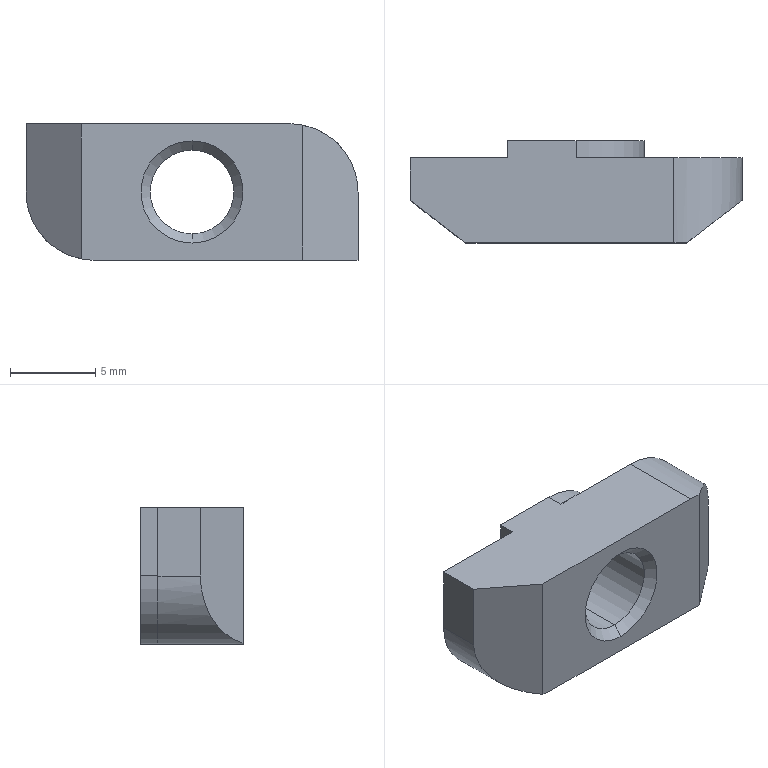Part | SolidWorks | features BaseBody 1 | 1 solid | 22 faces | box 19.5 x 6 x 8 mm | volume 631.457 mm3 | plane 12 | cylinder 6 | cone 4 | commonest cylinder face diameters 8 x4 4.917 x2
STEP:
#1=CARTESIAN_POINT('',(9.75,0.5415,-1.541));
#2=VERTEX_POINT('',#1);
#3=CARTESIAN_POINT('',(9.75,0.5415,-6.459));
#4=VERTEX_POINT('',#3);
#5=CARTESIAN_POINT('',(9.75,0.5415,-4.));
#6=DIRECTION('',(0.,-1.,0.));
#7=DIRECTION('',(0.,0.,-1.));
#8=AXIS2_PLACEMENT_3D('',#5,#6,#7);
#9=CIRCLE('',#8,2.459);
#10=EDGE_CURVE('',#2,#4,#9,.T.);
#11=ORIENTED_EDGE('',*,*,#10,.F.);
#12=CARTESIAN_POINT('',(9.75,0.,-1.));
#13=VERTEX_POINT('',#12);
#14=CARTESIAN_POINT('',(9.75,0.,-1.));
#15=DIRECTION('',(0.,-0.7071,0.7071));
#16=VECTOR('',#15,1000.);
#17=LINE('',#14,#16);
#18=EDGE_CURVE('',#2,#13,#17,.T.);
#19=ORIENTED_EDGE('',*,*,#18,.T.);
#20=CARTESIAN_POINT('',(9.75,0.,-7.));
#21=VERTEX_POINT('',#20);
#22=CARTESIAN_POINT('',(9.75,0.,-4.));
#23=DIRECTION('',(0.,-1.,0.));
#24=DIRECTION('',(0.,0.,-1.));
#25=AXIS2_PLACEMENT_3D('',#22,#23,#24);
#26=CIRCLE('',#25,3.);
#27=EDGE_CURVE('',#13,#21,#26,.T.);
#28=ORIENTED_EDGE('',*,*,#27,.T.);
#29=CARTESIAN_POINT('',(9.75,0.,-7.));
#30=DIRECTION('',(0.,-0.7071,-0.7071));
#31=VECTOR('',#30,1000.);
#32=LINE('',#29,#31);
#33=EDGE_CURVE('',#4,#21,#32,.T.);
#34=ORIENTED_EDGE('',*,*,#33,.F.);
#35=EDGE_LOOP('',(#11,#19,#28,#34));
#36=FACE_OUTER_BOUND('',#35,.T.);
#37=CARTESIAN_POINT('',(9.75,0.,-4.));
#38=DIRECTION('',(0.,-1.,0.));
#39=DIRECTION('',(0.,0.,-1.));
#40=AXIS2_PLACEMENT_3D('',#37,#38,#39);
#41=CONICAL_SURFACE('',#40,3.,0.7854);
#42=ADVANCED_FACE('',(#36),#41,.F.);
#43=CARTESIAN_POINT('',(9.75,5.459,-6.459));
#44=VERTEX_POINT('',#43);
#45=CARTESIAN_POINT('',(9.75,5.459,-1.541));
#46=VERTEX_POINT('',#45);
#47=CARTESIAN_POINT('',(9.75,5.459,-4.));
#48=DIRECTION('',(0.,1.,0.));
#49=DIRECTION('',(0.,0.,1.));
#50=AXIS2_PLACEMENT_3D('',#47,#48,#49);
#51=CIRCLE('',#50,2.459);
#52=EDGE_CURVE('',#44,#46,#51,.T.);
#53=ORIENTED_EDGE('',*,*,#52,.F.);
#54=CARTESIAN_POINT('',(9.75,6.,-7.));
#55=VERTEX_POINT('',#54);
#56=CARTESIAN_POINT('',(9.75,6.,-7.));
#57=DIRECTION('',(0.,0.7071,-0.7071));
#58=VECTOR('',#57,1000.);
#59=LINE('',#56,#58);
#60=EDGE_CURVE('',#44,#55,#59,.T.);
#61=ORIENTED_EDGE('',*,*,#60,.T.);
#62=CARTESIAN_POINT('',(9.75,6.,-1.));
#63=VERTEX_POINT('',#62);
#64=CARTESIAN_POINT('',(9.75,6.,-4.));
#65=DIRECTION('',(0.,-1.,0.));
#66=DIRECTION('',(0.,0.,1.));
#67=AXIS2_PLACEMENT_3D('',#64,#65,#66);
#68=CIRCLE('',#67,3.);
#69=EDGE_CURVE('',#63,#55,#68,.T.);
#70=ORIENTED_EDGE('',*,*,#69,.F.);
#71=CARTESIAN_POINT('',(9.75,6.,-1.));
#72=DIRECTION('',(0.,0.7071,0.7071));
#73=VECTOR('',#72,1000.);
#74=LINE('',#71,#73);
#75=EDGE_CURVE('',#46,#63,#74,.T.);
#76=ORIENTED_EDGE('',*,*,#75,.F.);
#77=EDGE_LOOP('',(#53,#61,#70,#76));
#78=FACE_OUTER_BOUND('',#77,.T.);
#79=CARTESIAN_POINT('',(9.75,6.,-4.));
#80=DIRECTION('',(0.,1.,0.));
#81=DIRECTION('',(0.,0.,1.));
#82=AXIS2_PLACEMENT_3D('',#79,#80,#81);
#83=CONICAL_SURFACE('',#82,3.,0.7854);
#84=ADVANCED_FACE('',(#78),#83,.F.);
#85=ORIENTED_EDGE('',*,*,#10,.T.);
#86=CARTESIAN_POINT('',(9.75,0.,-6.458));
#87=DIRECTION('',(0.,1.,0.));
#88=VECTOR('',#87,1000.);
#89=LINE('',#86,#88);
#90=EDGE_CURVE('',#4,#44,#89,.T.);
#91=ORIENTED_EDGE('',*,*,#90,.T.);
#92=ORIENTED_EDGE('',*,*,#52,.T.);
#93=CARTESIAN_POINT('',(9.75,0.,-1.542));
#94=DIRECTION('',(0.,1.,0.));
#95=VECTOR('',#94,1000.);
#96=LINE('',#93,#95);
#97=EDGE_CURVE('',#2,#46,#96,.T.);
#98=ORIENTED_EDGE('',*,*,#97,.F.);
#99=EDGE_LOOP('',(#85,#91,#92,#98));
#100=FACE_OUTER_BOUND('',#99,.T.);
#101=CARTESIAN_POINT('',(9.75,0.,-4.));
#102=DIRECTION('',(0.,1.,0.));
#103=DIRECTION('',(0.,0.,1.));
#104=AXIS2_PLACEMENT_3D('',#101,#102,#103);
#105=CYLINDRICAL_SURFACE('',#104,2.458);
#106=ADVANCED_FACE('',(#100),#105,.F.);
#107=CARTESIAN_POINT('',(3.25,0.,0.));
#108=VERTEX_POINT('',#107);
#109=CARTESIAN_POINT('',(0.,2.5,0.));
#110=VERTEX_POINT('',#109);
#111=CARTESIAN_POINT('',(3.25,0.,0.));
#112=DIRECTION('',(-0.7926,0.6097,0.));
#113=VECTOR('',#112,1000.);
#114=LINE('',#111,#113);
#115=EDGE_CURVE('',#108,#110,#114,.T.);
#116=ORIENTED_EDGE('',*,*,#115,.F.);
#117=CARTESIAN_POINT('',(15.5,0.,0.));
#118=VERTEX_POINT('',#117);
#119=CARTESIAN_POINT('',(0.,0.,0.));
#120=DIRECTION('',(-1.,0.,0.));
#121=VECTOR('',#120,1000.);
#122=LINE('',#119,#121);
#123=EDGE_CURVE('',#118,#108,#122,.T.);
#124=ORIENTED_EDGE('',*,*,#123,.F.);
#125=CARTESIAN_POINT('',(15.5,5.,0.));
#126=VERTEX_POINT('',#125);
#127=CARTESIAN_POINT('',(15.5,5.,0.));
#128=DIRECTION('',(0.,-1.,0.));
#129=VECTOR('',#128,1000.);
#130=LINE('',#127,#129);
#131=EDGE_CURVE('',#126,#118,#130,.T.);
#132=ORIENTED_EDGE('',*,*,#131,.F.);
#133=CARTESIAN_POINT('',(9.75,5.,0.));
#134=VERTEX_POINT('',#133);
#135=CARTESIAN_POINT('',(0.,5.,0.));
#136=DIRECTION('',(1.,0.,0.));
#137=VECTOR('',#136,1000.);
#138=LINE('',#135,#137);
#139=EDGE_CURVE('',#134,#126,#138,.T.);
#140=ORIENTED_EDGE('',*,*,#139,.F.);
#141=CARTESIAN_POINT('',(9.75,6.,0.));
#142=VERTEX_POINT('',#141);
#143=CARTESIAN_POINT('',(9.75,6.,0.));
#144=DIRECTION('',(0.,-1.,0.));
#145=VECTOR('',#144,1000.);
#146=LINE('',#143,#145);
#147=EDGE_CURVE('',#142,#134,#146,.T.);
#148=ORIENTED_EDGE('',*,*,#147,.F.);
#149=CARTESIAN_POINT('',(5.75,6.,0.));
#150=VERTEX_POINT('',#149);
#151=CARTESIAN_POINT('',(0.,6.,0.));
#152=DIRECTION('',(1.,0.,0.));
#153=VECTOR('',#152,1000.);
#154=LINE('',#151,#153);
#155=EDGE_CURVE('',#150,#142,#154,.T.);
#156=ORIENTED_EDGE('',*,*,#155,.F.);
#157=CARTESIAN_POINT('',(5.75,5.,0.));
#158=VERTEX_POINT('',#157);
#159=CARTESIAN_POINT('',(5.75,6.,0.));
#160=DIRECTION('',(0.,-1.,0.));
#161=VECTOR('',#160,1000.);
#162=LINE('',#159,#161);
#163=EDGE_CURVE('',#150,#158,#162,.T.);
#164=ORIENTED_EDGE('',*,*,#163,.T.);
#165=CARTESIAN_POINT('',(0.,5.,0.));
#166=VERTEX_POINT('',#165);
#167=CARTESIAN_POINT('',(0.,5.,0.));
#168=DIRECTION('',(1.,0.,0.));
#169=VECTOR('',#168,1000.);
#170=LINE('',#167,#169);
#171=EDGE_CURVE('',#166,#158,#170,.T.);
#172=ORIENTED_EDGE('',*,*,#171,.F.);
#173=CARTESIAN_POINT('',(0.,5.,0.));
#174=DIRECTION('',(0.,1.,0.));
#175=VECTOR('',#174,1000.);
#176=LINE('',#173,#175);
#177=EDGE_CURVE('',#110,#166,#176,.T.);
#178=ORIENTED_EDGE('',*,*,#177,.F.);
#179=EDGE_LOOP('',(#116,#124,#132,#140,#148,#156,#164,#172,#178));
#180=FACE_OUTER_BOUND('',#179,.T.);
#181=CARTESIAN_POINT('',(0.,5.,0.));
#182=DIRECTION('',(0.,0.,-1.));
#183=DIRECTION('',(-1.,0.,0.));
#184=AXIS2_PLACEMENT_3D('',#181,#182,#183);
#185=PLANE('',#184);
#186=ADVANCED_FACE('',(#180),#185,.F.);
#187=CARTESIAN_POINT('',(0.,2.5,-4.));
#188=VERTEX_POINT('',#187);
#189=CARTESIAN_POINT('',(0.,2.5,-4.));
#190=DIRECTION('',(0.,0.,-1.));
#191=VECTOR('',#190,1000.);
#192=LINE('',#189,#191);
#193=EDGE_CURVE('',#110,#188,#192,.T.);
#194=ORIENTED_EDGE('',*,*,#193,.F.);
#195=ORIENTED_EDGE('',*,*,#177,.T.);
#196=CARTESIAN_POINT('',(0.,5.,-4.));
#197=VERTEX_POINT('',#196);
#198=CARTESIAN_POINT('',(0.,5.,-4.));
#199=DIRECTION('',(0.,0.,1.));
#200=VECTOR('',#199,1000.);
#201=LINE('',#198,#200);
#202=EDGE_CURVE('',#197,#166,#201,.T.);
#203=ORIENTED_EDGE('',*,*,#202,.F.);
#204=CARTESIAN_POINT('',(0.,5.,-4.));
#205=DIRECTION('',(0.,1.,0.));
#206=VECTOR('',#205,1000.);
#207=LINE('',#204,#206);
#208=EDGE_CURVE('',#188,#197,#207,.T.);
#209=ORIENTED_EDGE('',*,*,#208,.F.);
#210=EDGE_LOOP('',(#194,#195,#203,#209));
#211=FACE_OUTER_BOUND('',#210,.T.);
#212=CARTESIAN_POINT('',(0.,5.,-4.));
#213=DIRECTION('',(1.,0.,0.));
#214=DIRECTION('',(0.,0.,-1.));
#215=AXIS2_PLACEMENT_3D('',#212,#213,#214);
#216=PLANE('',#215);
#217=ADVANCED_FACE('',(#211),#216,.F.);
#218=ORIENTED_EDGE('',*,*,#115,.T.);
#219=ORIENTED_EDGE('',*,*,#193,.T.);
#220=CARTESIAN_POINT('',(3.25,0.,-7.929));
#221=VERTEX_POINT('',#220);
#222=CARTESIAN_POINT('',(3.25,0.,-7.929));
#223=CARTESIAN_POINT('',(1.279,1.516,-7.553));
#224=CARTESIAN_POINT('',(0.,2.5,-6.007));
#225=CARTESIAN_POINT('',(0.,2.5,-4.));
#226=(BOUNDED_CURVE()B_SPLINE_CURVE(3,(#222,#223,#224,#225),.UNSPECIFIED.,.F.,.F.)B_SPLINE_CURVE_WITH_KNOTS((4,4),(4.901,6.283),.UNSPECIFIED.)CURVE()GEOMETRIC_REPRESENTATION_ITEM()RATIONAL_B_SPLINE_CURVE((1.,0.847,0.847,1.))REPRESENTATION_ITEM(''));
#227=EDGE_CURVE('',#221,#188,#226,.T.);
#228=ORIENTED_EDGE('',*,*,#227,.F.);
#229=CARTESIAN_POINT('',(3.25,0.,-10.));
#230=DIRECTION('',(0.,0.,-1.));
#231=VECTOR('',#230,1000.);
#232=LINE('',#229,#231);
#233=EDGE_CURVE('',#108,#221,#232,.T.);
#234=ORIENTED_EDGE('',*,*,#233,.F.);
#235=EDGE_LOOP('',(#218,#219,#228,#234));
#236=FACE_OUTER_BOUND('',#235,.T.);
#237=CARTESIAN_POINT('',(3.25,0.,-10.));
#238=DIRECTION('',(0.6097,0.7926,0.));
#239=DIRECTION('',(-0.7926,0.6097,0.));
#240=AXIS2_PLACEMENT_3D('',#237,#238,#239);
#241=PLANE('',#240);
#242=ADVANCED_FACE('',(#236),#241,.F.);
#243=CARTESIAN_POINT('',(9.75,0.,-4.));
#244=DIRECTION('',(0.,-1.,0.));
#245=DIRECTION('',(0.,0.,-1.));
#246=AXIS2_PLACEMENT_3D('',#243,#244,#245);
#247=CIRCLE('',#246,3.);
#248=EDGE_CURVE('',#21,#13,#247,.T.);
#249=ORIENTED_EDGE('',*,*,#248,.F.);
#250=ORIENTED_EDGE('',*,*,#27,.F.);
#251=EDGE_LOOP('',(#249,#250));
#252=FACE_BOUND('',#251,.T.);
#253=CARTESIAN_POINT('',(16.25,0.,-0.07094));
#254=VERTEX_POINT('',#253);
#255=CARTESIAN_POINT('',(16.25,0.,-8.));
#256=VERTEX_POINT('',#255);
#257=CARTESIAN_POINT('',(16.25,0.,-4.));
#258=DIRECTION('',(0.,0.,-1.));
#259=VECTOR('',#258,1000.);
#260=LINE('',#257,#259);
#261=EDGE_CURVE('',#254,#256,#260,.T.);
#262=ORIENTED_EDGE('',*,*,#261,.F.);
#263=CARTESIAN_POINT('',(15.5,0.,-4.));
#264=DIRECTION('',(0.,1.,0.));
#265=DIRECTION('',(0.,0.,1.));
#266=AXIS2_PLACEMENT_3D('',#263,#264,#265);
#267=CIRCLE('',#266,4.);
#268=EDGE_CURVE('',#118,#254,#267,.T.);
#269=ORIENTED_EDGE('',*,*,#268,.F.);
#270=ORIENTED_EDGE('',*,*,#123,.T.);
#271=ORIENTED_EDGE('',*,*,#233,.T.);
#272=CARTESIAN_POINT('',(4.,0.,-8.));
#273=VERTEX_POINT('',#272);
#274=CARTESIAN_POINT('',(4.,0.,-4.));
#275=DIRECTION('',(0.,1.,0.));
#276=DIRECTION('',(0.,0.,1.));
#277=AXIS2_PLACEMENT_3D('',#274,#275,#276);
#278=CIRCLE('',#277,4.);
#279=EDGE_CURVE('',#273,#221,#278,.T.);
#280=ORIENTED_EDGE('',*,*,#279,.F.);
#281=CARTESIAN_POINT('',(15.5,0.,-8.));
#282=DIRECTION('',(-1.,0.,0.));
#283=VECTOR('',#282,1000.);
#284=LINE('',#281,#283);
#285=EDGE_CURVE('',#256,#273,#284,.T.);
#286=ORIENTED_EDGE('',*,*,#285,.F.);
#287=EDGE_LOOP('',(#262,#269,#270,#271,#280,#286));
#288=FACE_OUTER_BOUND('',#287,.T.);
#289=CARTESIAN_POINT('',(15.5,0.,-4.));
#290=DIRECTION('',(0.,1.,0.));
#291=DIRECTION('',(0.,0.,1.));
#292=AXIS2_PLACEMENT_3D('',#289,#290,#291);
#293=PLANE('',#292);
#294=ADVANCED_FACE('',(#252,#288),#293,.F.);
#295=CARTESIAN_POINT('',(19.5,5.,-4.));
#296=VERTEX_POINT('',#295);
#297=CARTESIAN_POINT('',(15.5,5.,-4.));
#298=DIRECTION('',(0.,-1.,0.));
#299=DIRECTION('',(0.,0.,1.));
#300=AXIS2_PLACEMENT_3D('',#297,#298,#299);
#301=CIRCLE('',#300,4.);
#302=EDGE_CURVE('',#296,#126,#301,.T.);
#303=ORIENTED_EDGE('',*,*,#302,.T.);
#304=ORIENTED_EDGE('',*,*,#131,.T.);
#305=ORIENTED_EDGE('',*,*,#268,.T.);
#306=CARTESIAN_POINT('',(19.5,2.5,-4.));
#307=VERTEX_POINT('',#306);
#308=CARTESIAN_POINT('',(16.25,0.,-0.07094));
#309=CARTESIAN_POINT('',(18.221,1.516,-0.4472));
#310=CARTESIAN_POINT('',(19.5,2.5,-1.993));
#311=CARTESIAN_POINT('',(19.5,2.5,-4.));
#312=(BOUNDED_CURVE()B_SPLINE_CURVE(3,(#308,#309,#310,#311),.UNSPECIFIED.,.F.,.T.)B_SPLINE_CURVE_WITH_KNOTS((4,4),(4.901,6.283),.UNSPECIFIED.)CURVE()GEOMETRIC_REPRESENTATION_ITEM()RATIONAL_B_SPLINE_CURVE((1.,0.847,0.847,1.))REPRESENTATION_ITEM(''));
#313=EDGE_CURVE('',#254,#307,#312,.T.);
#314=ORIENTED_EDGE('',*,*,#313,.T.);
#315=CARTESIAN_POINT('',(19.5,5.,-4.));
#316=DIRECTION('',(0.,1.,0.));
#317=VECTOR('',#316,1000.);
#318=LINE('',#315,#317);
#319=EDGE_CURVE('',#307,#296,#318,.T.);
#320=ORIENTED_EDGE('',*,*,#319,.T.);
#321=EDGE_LOOP('',(#303,#304,#305,#314,#320));
#322=FACE_OUTER_BOUND('',#321,.T.);
#323=CARTESIAN_POINT('',(15.5,5.,-4.));
#324=DIRECTION('',(0.,1.,0.));
#325=DIRECTION('',(0.,0.,1.));
#326=AXIS2_PLACEMENT_3D('',#323,#324,#325);
#327=CYLINDRICAL_SURFACE('',#326,4.);
#328=ADVANCED_FACE('',(#322),#327,.T.);
#329=CARTESIAN_POINT('',(19.5,5.,-8.));
#330=VERTEX_POINT('',#329);
#331=CARTESIAN_POINT('',(19.5,5.,-4.));
#332=DIRECTION('',(0.,0.,-1.));
#333=VECTOR('',#332,1000.);
#334=LINE('',#331,#333);
#335=EDGE_CURVE('',#296,#330,#334,.T.);
#336=ORIENTED_EDGE('',*,*,#335,.T.);
#337=CARTESIAN_POINT('',(13.75,5.,-8.));
#338=VERTEX_POINT('',#337);
#339=CARTESIAN_POINT('',(15.5,5.,-8.));
#340=DIRECTION('',(-1.,0.,0.));
#341=VECTOR('',#340,1000.);
#342=LINE('',#339,#341);
#343=EDGE_CURVE('',#330,#338,#342,.T.);
#344=ORIENTED_EDGE('',*,*,#343,.T.);
#345=CARTESIAN_POINT('',(13.75,5.,-4.));
#346=VERTEX_POINT('',#345);
#347=CARTESIAN_POINT('',(13.75,5.,-4.));
#348=DIRECTION('',(0.,0.,1.));
#349=VECTOR('',#348,1000.);
#350=LINE('',#347,#349);
#351=EDGE_CURVE('',#338,#346,#350,.T.);
#352=ORIENTED_EDGE('',*,*,#351,.T.);
#353=CARTESIAN_POINT('',(9.75,5.,-4.));
#354=DIRECTION('',(0.,-1.,0.));
#355=DIRECTION('',(0.,0.,1.));
#356=AXIS2_PLACEMENT_3D('',#353,#354,#355);
#357=CIRCLE('',#356,4.);
#358=EDGE_CURVE('',#346,#134,#357,.T.);
#359=ORIENTED_EDGE('',*,*,#358,.T.);
#360=ORIENTED_EDGE('',*,*,#139,.T.);
#361=ORIENTED_EDGE('',*,*,#302,.F.);
#362=EDGE_LOOP('',(#336,#344,#352,#359,#360,#361));
#363=FACE_OUTER_BOUND('',#362,.T.);
#364=CARTESIAN_POINT('',(15.5,5.,-4.));
#365=DIRECTION('',(0.,1.,0.));
#366=DIRECTION('',(0.,0.,1.));
#367=AXIS2_PLACEMENT_3D('',#364,#365,#366);
#368=PLANE('',#367);
#369=ADVANCED_FACE('',(#363),#368,.T.);
#370=ORIENTED_EDGE('',*,*,#69,.T.);
#371=CARTESIAN_POINT('',(9.75,6.,-4.));
#372=DIRECTION('',(0.,-1.,0.));
#373=DIRECTION('',(0.,0.,1.));
#374=AXIS2_PLACEMENT_3D('',#371,#372,#373);
#375=CIRCLE('',#374,3.);
#376=EDGE_CURVE('',#55,#63,#375,.T.);
#377=ORIENTED_EDGE('',*,*,#376,.T.);
#378=EDGE_LOOP('',(#370,#377));
#379=FACE_BOUND('',#378,.T.);
#380=CARTESIAN_POINT('',(13.75,6.,-8.));
#381=VERTEX_POINT('',#380);
#382=CARTESIAN_POINT('',(9.75,6.,-8.));
#383=VERTEX_POINT('',#382);
#384=CARTESIAN_POINT('',(9.75,6.,-8.));
#385=DIRECTION('',(-1.,0.,0.));
#386=VECTOR('',#385,1000.);
#387=LINE('',#384,#386);
#388=EDGE_CURVE('',#381,#383,#387,.T.);
#389=ORIENTED_EDGE('',*,*,#388,.T.);
#390=CARTESIAN_POINT('',(5.75,6.,-4.));
#391=VERTEX_POINT('',#390);
#392=CARTESIAN_POINT('',(9.75,6.,-4.));
#393=DIRECTION('',(0.,1.,0.));
#394=DIRECTION('',(0.,0.,1.));
#395=AXIS2_PLACEMENT_3D('',#392,#393,#394);
#396=CIRCLE('',#395,4.);
#397=EDGE_CURVE('',#383,#391,#396,.T.);
#398=ORIENTED_EDGE('',*,*,#397,.T.);
#399=CARTESIAN_POINT('',(5.75,6.,-4.));
#400=DIRECTION('',(0.,0.,1.));
#401=VECTOR('',#400,1000.);
#402=LINE('',#399,#401);
#403=EDGE_CURVE('',#391,#150,#402,.T.);
#404=ORIENTED_EDGE('',*,*,#403,.T.);
#405=ORIENTED_EDGE('',*,*,#155,.T.);
#406=CARTESIAN_POINT('',(13.75,6.,-4.));
#407=VERTEX_POINT('',#406);
#408=CARTESIAN_POINT('',(9.75,6.,-4.));
#409=DIRECTION('',(0.,1.,0.));
#410=DIRECTION('',(0.,0.,1.));
#411=AXIS2_PLACEMENT_3D('',#408,#409,#410);
#412=CIRCLE('',#411,4.);
#413=EDGE_CURVE('',#142,#407,#412,.T.);
#414=ORIENTED_EDGE('',*,*,#413,.T.);
#415=CARTESIAN_POINT('',(13.75,6.,-4.));
#416=DIRECTION('',(0.,0.,-1.));
#417=VECTOR('',#416,1000.);
#418=LINE('',#415,#417);
#419=EDGE_CURVE('',#407,#381,#418,.T.);
#420=ORIENTED_EDGE('',*,*,#419,.T.);
#421=EDGE_LOOP('',(#389,#398,#404,#405,#414,#420));
#422=FACE_OUTER_BOUND('',#421,.T.);
#423=CARTESIAN_POINT('',(9.75,6.,-4.));
#424=DIRECTION('',(0.,1.,0.));
#425=DIRECTION('',(0.,0.,1.));
#426=AXIS2_PLACEMENT_3D('',#423,#424,#425);
#427=PLANE('',#426);
#428=ADVANCED_FACE('',(#379,#422),#427,.T.);
#429=ORIENTED_EDGE('',*,*,#202,.T.);
#430=ORIENTED_EDGE('',*,*,#171,.T.);
#431=CARTESIAN_POINT('',(5.75,5.,-4.));
#432=VERTEX_POINT('',#431);
#433=CARTESIAN_POINT('',(5.75,5.,-4.));
#434=DIRECTION('',(0.,0.,-1.));
#435=VECTOR('',#434,1000.);
#436=LINE('',#433,#435);
#437=EDGE_CURVE('',#158,#432,#436,.T.);
#438=ORIENTED_EDGE('',*,*,#437,.T.);
#439=CARTESIAN_POINT('',(9.75,5.,-8.));
#440=VERTEX_POINT('',#439);
#441=CARTESIAN_POINT('',(9.75,5.,-4.));
#442=DIRECTION('',(0.,-1.,0.));
#443=DIRECTION('',(0.,0.,1.));
#444=AXIS2_PLACEMENT_3D('',#441,#442,#443);
#445=CIRCLE('',#444,4.);
#446=EDGE_CURVE('',#432,#440,#445,.T.);
#447=ORIENTED_EDGE('',*,*,#446,.T.);
#448=CARTESIAN_POINT('',(4.,5.,-8.));
#449=VERTEX_POINT('',#448);
#450=CARTESIAN_POINT('',(15.5,5.,-8.));
#451=DIRECTION('',(-1.,0.,0.));
#452=VECTOR('',#451,1000.);
#453=LINE('',#450,#452);
#454=EDGE_CURVE('',#440,#449,#453,.T.);
#455=ORIENTED_EDGE('',*,*,#454,.T.);
#456=CARTESIAN_POINT('',(4.,5.,-4.));
#457=DIRECTION('',(0.,1.,0.));
#458=DIRECTION('',(0.,0.,1.));
#459=AXIS2_PLACEMENT_3D('',#456,#457,#458);
#460=CIRCLE('',#459,4.);
#461=EDGE_CURVE('',#449,#197,#460,.T.);
#462=ORIENTED_EDGE('',*,*,#461,.T.);
#463=EDGE_LOOP('',(#429,#430,#438,#447,#455,#462));
#464=FACE_OUTER_BOUND('',#463,.T.);
#465=CARTESIAN_POINT('',(15.5,5.,-4.));
#466=DIRECTION('',(0.,1.,0.));
#467=DIRECTION('',(0.,0.,1.));
#468=AXIS2_PLACEMENT_3D('',#465,#466,#467);
#469=PLANE('',#468);
#470=ADVANCED_FACE('',(#464),#469,.T.);
#471=ORIENTED_EDGE('',*,*,#461,.F.);
#472=CARTESIAN_POINT('',(4.,5.,-8.));
#473=DIRECTION('',(0.,-1.,0.));
#474=VECTOR('',#473,1000.);
#475=LINE('',#472,#474);
#476=EDGE_CURVE('',#449,#273,#475,.T.);
#477=ORIENTED_EDGE('',*,*,#476,.T.);
#478=ORIENTED_EDGE('',*,*,#279,.T.);
#479=ORIENTED_EDGE('',*,*,#227,.T.);
#480=ORIENTED_EDGE('',*,*,#208,.T.);
#481=EDGE_LOOP('',(#471,#477,#478,#479,#480));
#482=FACE_OUTER_BOUND('',#481,.T.);
#483=CARTESIAN_POINT('',(4.,5.,-4.));
#484=DIRECTION('',(0.,1.,0.));
#485=DIRECTION('',(0.,0.,1.));
#486=AXIS2_PLACEMENT_3D('',#483,#484,#485);
#487=CYLINDRICAL_SURFACE('',#486,4.);
#488=ADVANCED_FACE('',(#482),#487,.T.);
#489=ORIENTED_EDGE('',*,*,#18,.F.);
#490=CARTESIAN_POINT('',(9.75,0.5415,-4.));
#491=DIRECTION('',(0.,-1.,0.));
#492=DIRECTION('',(0.,0.,-1.));
#493=AXIS2_PLACEMENT_3D('',#490,#491,#492);
#494=CIRCLE('',#493,2.459);
#495=EDGE_CURVE('',#4,#2,#494,.T.);
#496=ORIENTED_EDGE('',*,*,#495,.F.);
#497=ORIENTED_EDGE('',*,*,#33,.T.);
#498=ORIENTED_EDGE('',*,*,#248,.T.);
#499=EDGE_LOOP('',(#489,#496,#497,#498));
#500=FACE_OUTER_BOUND('',#499,.T.);
#501=CARTESIAN_POINT('',(9.75,0.,-4.));
#502=DIRECTION('',(0.,-1.,0.));
#503=DIRECTION('',(0.,0.,-1.));
#504=AXIS2_PLACEMENT_3D('',#501,#502,#503);
#505=CONICAL_SURFACE('',#504,3.,0.7854);
#506=ADVANCED_FACE('',(#500),#505,.F.);
#507=CARTESIAN_POINT('',(19.5,2.5,-8.));
#508=VERTEX_POINT('',#507);
#509=CARTESIAN_POINT('',(16.25,0.,-8.));
#510=DIRECTION('',(0.7926,0.6097,0.));
#511=VECTOR('',#510,1000.);
#512=LINE('',#509,#511);
#513=EDGE_CURVE('',#256,#508,#512,.T.);
#514=ORIENTED_EDGE('',*,*,#513,.F.);
#515=ORIENTED_EDGE('',*,*,#285,.T.);
#516=ORIENTED_EDGE('',*,*,#476,.F.);
#517=ORIENTED_EDGE('',*,*,#454,.F.);
#518=CARTESIAN_POINT('',(9.75,5.,-8.));
#519=DIRECTION('',(0.,-1.,0.));
#520=VECTOR('',#519,1000.);
#521=LINE('',#518,#520);
#522=EDGE_CURVE('',#383,#440,#521,.T.);
#523=ORIENTED_EDGE('',*,*,#522,.F.);
#524=ORIENTED_EDGE('',*,*,#388,.F.);
#525=CARTESIAN_POINT('',(13.75,5.,-8.));
#526=DIRECTION('',(0.,1.,0.));
#527=VECTOR('',#526,1000.);
#528=LINE('',#525,#527);
#529=EDGE_CURVE('',#338,#381,#528,.T.);
#530=ORIENTED_EDGE('',*,*,#529,.F.);
#531=ORIENTED_EDGE('',*,*,#343,.F.);
#532=CARTESIAN_POINT('',(19.5,5.,-8.));
#533=DIRECTION('',(0.,1.,0.));
#534=VECTOR('',#533,1000.);
#535=LINE('',#532,#534);
#536=EDGE_CURVE('',#508,#330,#535,.T.);
#537=ORIENTED_EDGE('',*,*,#536,.F.);
#538=EDGE_LOOP('',(#514,#515,#516,#517,#523,#524,#530,#531,#537));
#539=FACE_OUTER_BOUND('',#538,.T.);
#540=CARTESIAN_POINT('',(19.5,5.,-8.));
#541=DIRECTION('',(0.,0.,1.));
#542=DIRECTION('',(1.,0.,0.));
#543=AXIS2_PLACEMENT_3D('',#540,#541,#542);
#544=PLANE('',#543);
#545=ADVANCED_FACE('',(#539),#544,.F.);
#546=ORIENTED_EDGE('',*,*,#513,.T.);
#547=CARTESIAN_POINT('',(19.5,2.5,-10.));
#548=DIRECTION('',(0.,0.,-1.));
#549=VECTOR('',#548,1000.);
#550=LINE('',#547,#549);
#551=EDGE_CURVE('',#307,#508,#550,.T.);
#552=ORIENTED_EDGE('',*,*,#551,.F.);
#553=ORIENTED_EDGE('',*,*,#313,.F.);
#554=ORIENTED_EDGE('',*,*,#261,.T.);
#555=EDGE_LOOP('',(#546,#552,#553,#554));
#556=FACE_OUTER_BOUND('',#555,.T.);
#557=CARTESIAN_POINT('',(19.5,2.5,-10.));
#558=DIRECTION('',(-0.6097,0.7926,0.));
#559=DIRECTION('',(-0.7926,-0.6097,0.));
#560=AXIS2_PLACEMENT_3D('',#557,#558,#559);
#561=PLANE('',#560);
#562=ADVANCED_FACE('',(#556),#561,.F.);
#563=ORIENTED_EDGE('',*,*,#551,.T.);
#564=ORIENTED_EDGE('',*,*,#536,.T.);
#565=ORIENTED_EDGE('',*,*,#335,.F.);
#566=ORIENTED_EDGE('',*,*,#319,.F.);
#567=EDGE_LOOP('',(#563,#564,#565,#566));
#568=FACE_OUTER_BOUND('',#567,.T.);
#569=CARTESIAN_POINT('',(19.5,5.,-4.));
#570=DIRECTION('',(-1.,0.,0.));
#571=DIRECTION('',(0.,0.,1.));
#572=AXIS2_PLACEMENT_3D('',#569,#570,#571);
#573=PLANE('',#572);
#574=ADVANCED_FACE('',(#568),#573,.F.);
#575=ORIENTED_EDGE('',*,*,#413,.F.);
#576=ORIENTED_EDGE('',*,*,#147,.T.);
#577=ORIENTED_EDGE('',*,*,#358,.F.);
#578=CARTESIAN_POINT('',(13.75,6.,-4.));
#579=DIRECTION('',(0.,1.,0.));
#580=VECTOR('',#579,1000.);
#581=LINE('',#578,#580);
#582=EDGE_CURVE('',#346,#407,#581,.T.);
#583=ORIENTED_EDGE('',*,*,#582,.T.);
#584=EDGE_LOOP('',(#575,#576,#577,#583));
#585=FACE_OUTER_BOUND('',#584,.T.);
#586=CARTESIAN_POINT('',(9.75,6.,-4.));
#587=DIRECTION('',(0.,1.,0.));
#588=DIRECTION('',(0.,0.,1.));
#589=AXIS2_PLACEMENT_3D('',#586,#587,#588);
#590=CYLINDRICAL_SURFACE('',#589,4.);
#591=ADVANCED_FACE('',(#585),#590,.T.);
#592=ORIENTED_EDGE('',*,*,#529,.T.);
#593=ORIENTED_EDGE('',*,*,#419,.F.);
#594=ORIENTED_EDGE('',*,*,#582,.F.);
#595=ORIENTED_EDGE('',*,*,#351,.F.);
#596=EDGE_LOOP('',(#592,#593,#594,#595));
#597=FACE_OUTER_BOUND('',#596,.T.);
#598=CARTESIAN_POINT('',(13.75,6.,-4.));
#599=DIRECTION('',(-1.,0.,0.));
#600=DIRECTION('',(0.,0.,1.));
#601=AXIS2_PLACEMENT_3D('',#598,#599,#600);
#602=PLANE('',#601);
#603=ADVANCED_FACE('',(#597),#602,.F.);
#604=ORIENTED_EDGE('',*,*,#60,.F.);
#605=CARTESIAN_POINT('',(9.75,5.459,-4.));
#606=DIRECTION('',(0.,1.,0.));
#607=DIRECTION('',(0.,0.,1.));
#608=AXIS2_PLACEMENT_3D('',#605,#606,#607);
#609=CIRCLE('',#608,2.459);
#610=EDGE_CURVE('',#46,#44,#609,.T.);
#611=ORIENTED_EDGE('',*,*,#610,.F.);
#612=ORIENTED_EDGE('',*,*,#75,.T.);
#613=ORIENTED_EDGE('',*,*,#376,.F.);
#614=EDGE_LOOP('',(#604,#611,#612,#613));
#615=FACE_OUTER_BOUND('',#614,.T.);
#616=CARTESIAN_POINT('',(9.75,6.,-4.));
#617=DIRECTION('',(0.,1.,0.));
#618=DIRECTION('',(0.,0.,1.));
#619=AXIS2_PLACEMENT_3D('',#616,#617,#618);
#620=CONICAL_SURFACE('',#619,3.,0.7854);
#621=ADVANCED_FACE('',(#615),#620,.F.);
#622=ORIENTED_EDGE('',*,*,#397,.F.);
#623=ORIENTED_EDGE('',*,*,#522,.T.);
#624=ORIENTED_EDGE('',*,*,#446,.F.);
#625=CARTESIAN_POINT('',(5.75,6.,-4.));
#626=DIRECTION('',(0.,1.,0.));
#627=VECTOR('',#626,1000.);
#628=LINE('',#625,#627);
#629=EDGE_CURVE('',#432,#391,#628,.T.);
#630=ORIENTED_EDGE('',*,*,#629,.T.);
#631=EDGE_LOOP('',(#622,#623,#624,#630));
#632=FACE_OUTER_BOUND('',#631,.T.);
#633=CARTESIAN_POINT('',(9.75,6.,-4.));
#634=DIRECTION('',(0.,1.,0.));
#635=DIRECTION('',(0.,0.,1.));
#636=AXIS2_PLACEMENT_3D('',#633,#634,#635);
#637=CYLINDRICAL_SURFACE('',#636,4.);
#638=ADVANCED_FACE('',(#632),#637,.T.);
#639=ORIENTED_EDGE('',*,*,#163,.F.);
#640=ORIENTED_EDGE('',*,*,#403,.F.);
#641=ORIENTED_EDGE('',*,*,#629,.F.);
#642=ORIENTED_EDGE('',*,*,#437,.F.);
#643=EDGE_LOOP('',(#639,#640,#641,#642));
#644=FACE_OUTER_BOUND('',#643,.T.);
#645=CARTESIAN_POINT('',(5.75,6.,-4.));
#646=DIRECTION('',(1.,0.,0.));
#647=DIRECTION('',(0.,0.,-1.));
#648=AXIS2_PLACEMENT_3D('',#645,#646,#647);
#649=PLANE('',#648);
#650=ADVANCED_FACE('',(#644),#649,.F.);
#651=ORIENTED_EDGE('',*,*,#90,.F.);
#652=ORIENTED_EDGE('',*,*,#495,.T.);
#653=ORIENTED_EDGE('',*,*,#97,.T.);
#654=ORIENTED_EDGE('',*,*,#610,.T.);
#655=EDGE_LOOP('',(#651,#652,#653,#654));
#656=FACE_OUTER_BOUND('',#655,.T.);
#657=CARTESIAN_POINT('',(9.75,0.,-4.));
#658=DIRECTION('',(0.,1.,0.));
#659=DIRECTION('',(0.,0.,1.));
#660=AXIS2_PLACEMENT_3D('',#657,#658,#659);
#661=CYLINDRICAL_SURFACE('',#660,2.458);
#662=ADVANCED_FACE('',(#656),#661,.F.);
#663=CLOSED_SHELL('',(#42,#84,#106,#186,#217,#242,#294,#328,#369,#428,#470,#488,#506,#545,#562,#574,#591,#603,#621,#638,#650,#662));
#664=MANIFOLD_SOLID_BREP('',#663);
#665=CARTESIAN_POINT('',(0.,0.,0.));
#666=DIRECTION('',(0.,0.,1.));
#667=DIRECTION('',(1.,0.,0.));
#668=AXIS2_PLACEMENT_3D('',#665,#666,#667);
#669=(LENGTH_UNIT()NAMED_UNIT(*)SI_UNIT(.MILLI.,.METRE.));
#670=UNCERTAINTY_MEASURE_WITH_UNIT(LENGTH_MEASURE(0.00001),#669,'','');
#671=(NAMED_UNIT(*)PLANE_ANGLE_UNIT()SI_UNIT($,.RADIAN.));
#672=(NAMED_UNIT(*)SI_UNIT($,.STERADIAN.)SOLID_ANGLE_UNIT());
#673=(GEOMETRIC_REPRESENTATION_CONTEXT(3)GLOBAL_UNCERTAINTY_ASSIGNED_CONTEXT((#670))GLOBAL_UNIT_ASSIGNED_CONTEXT((#669,#671,#672))REPRESENTATION_CONTEXT('',''));
#674=ADVANCED_BREP_SHAPE_REPRESENTATION('',(#664,#668),#673);